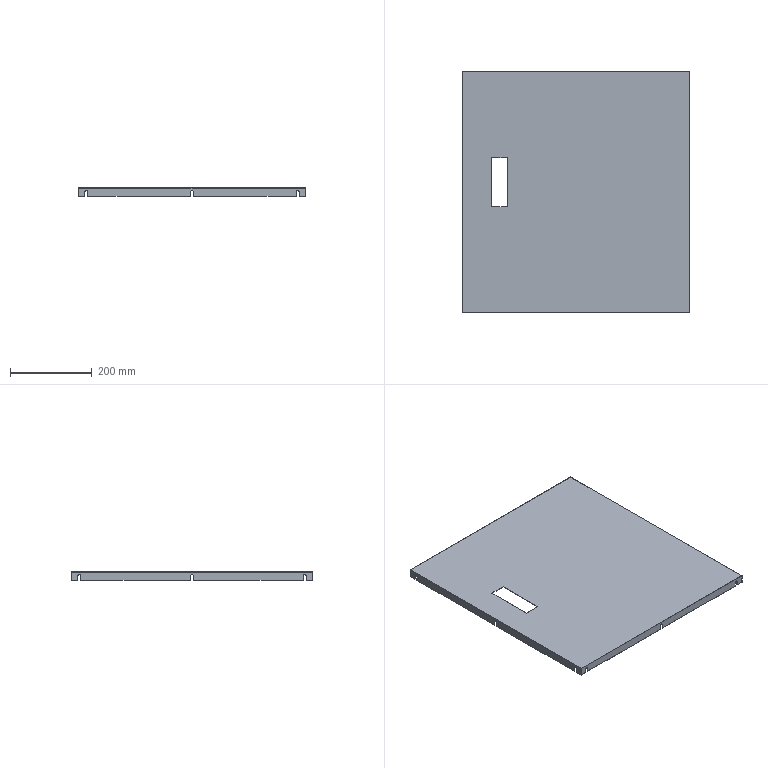Part | STEP file | 1 solid | 68 faces | box 558 x 593 x 20 mm | volume 368788 mm3 | plane 50 | cylinder 18 | commonest cylinder face diameters 7 x18